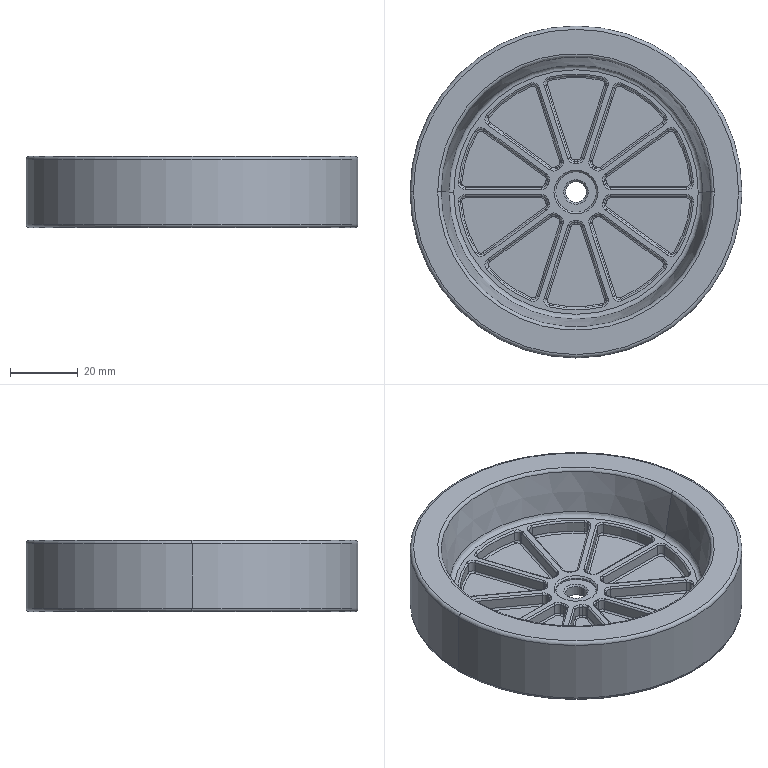Part | SolidWorks | features ICE 6, Fillet 5, Chamfer 2, CirPattern 1, Extrusion 1 | 1 solid | 307 faces | box 98 x 98 x 21 mm | volume 76167 mm3 | torus 148 | cylinder 118 | plane 35 | cone 6 | commonest cylinder face diameters 3 x50 1 x40 18 x10 68.71 x10 6.2 x2 12 x2